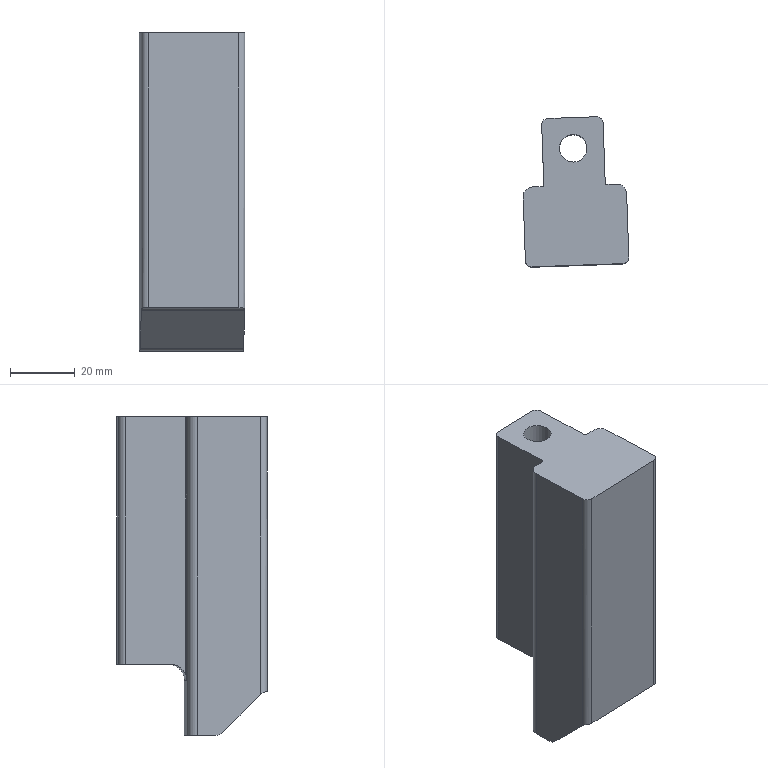Part | NX | features PU-10 2 | 1 solid | 25 faces | box 32.67 x 46.387 x 98.419 mm | volume 98260 mm3 | cylinder 13 | plane 12 | commonest cylinder face diameters 4 x4 6 x4 1 x2 8.506 x1 10 x1 14.5 x1
STEP:
#1=CARTESIAN_POINT('',(3512.219,-784.938,945.716));
#2=VERTEX_POINT('',#1);
#3=CARTESIAN_POINT('',(3512.07,-780.688,945.716));
#4=DIRECTION('',(0.,0.,-1.));
#5=DIRECTION('',(0.0349,-0.9994,0.));
#6=AXIS2_PLACEMENT_3D('',#3,#4,#5);
#7=CIRCLE('',#6,4.253);
#8=EDGE_CURVE('',#2,#2,#7,.F.);
#9=ORIENTED_EDGE('',*,*,#8,.T.);
#10=EDGE_LOOP('',(#9));
#11=FACE_BOUND('',#10,.T.);
#12=CARTESIAN_POINT('',(3511.922,-776.437,884.216));
#13=VERTEX_POINT('',#12);
#14=CARTESIAN_POINT('',(3512.07,-780.688,884.216));
#15=DIRECTION('',(0.,0.,1.));
#16=DIRECTION('',(1.,0.,0.));
#17=AXIS2_PLACEMENT_3D('',#14,#15,#16);
#18=CIRCLE('',#17,4.253);
#19=EDGE_CURVE('',#13,#13,#18,.T.);
#20=ORIENTED_EDGE('',*,*,#19,.F.);
#21=EDGE_LOOP('',(#20));
#22=FACE_BOUND('',#21,.T.);
#23=CARTESIAN_POINT('',(3512.07,-780.688,947.216));
#24=DIRECTION('',(0.,0.,-1.));
#25=DIRECTION('',(-0.0349,0.9994,0.));
#26=AXIS2_PLACEMENT_3D('',#23,#24,#25);
#27=CYLINDRICAL_SURFACE('',#26,4.253);
#28=ADVANCED_FACE('',(#11,#22),#27,.F.);
#29=CARTESIAN_POINT('',(3525.464,-791.727,945.716));
#30=VERTEX_POINT('',#29);
#31=CARTESIAN_POINT('',(3522.466,-791.832,945.716));
#32=VERTEX_POINT('',#31);
#33=CARTESIAN_POINT('',(3526.198,-791.701,945.716));
#34=DIRECTION('',(-0.9994,-0.0349,0.));
#35=VECTOR('',#34,1000.);
#36=LINE('',#33,#35);
#37=EDGE_CURVE('',#30,#32,#36,.T.);
#38=ORIENTED_EDGE('',*,*,#37,.T.);
#39=CARTESIAN_POINT('',(3521.948,-791.349,945.716));
#40=VERTEX_POINT('',#39);
#41=CARTESIAN_POINT('',(3522.448,-791.332,945.716));
#42=DIRECTION('',(0.,0.,-1.));
#43=DIRECTION('',(0.0349,-0.9994,0.));
#44=AXIS2_PLACEMENT_3D('',#41,#42,#43);
#45=CIRCLE('',#44,0.5);
#46=EDGE_CURVE('',#32,#40,#45,.T.);
#47=ORIENTED_EDGE('',*,*,#46,.T.);
#48=CARTESIAN_POINT('',(3521.303,-772.861,945.716));
#49=VERTEX_POINT('',#48);
#50=CARTESIAN_POINT('',(3521.966,-791.849,945.716));
#51=DIRECTION('',(0.0349,-0.9994,0.));
#52=VECTOR('',#51,1000.);
#53=LINE('',#50,#52);
#54=EDGE_CURVE('',#49,#40,#53,.T.);
#55=ORIENTED_EDGE('',*,*,#54,.F.);
#56=CARTESIAN_POINT('',(3519.234,-770.932,945.716));
#57=VERTEX_POINT('',#56);
#58=CARTESIAN_POINT('',(3519.304,-772.93,945.716));
#59=DIRECTION('',(0.,0.,-1.));
#60=DIRECTION('',(0.0349,-0.9994,0.));
#61=AXIS2_PLACEMENT_3D('',#58,#59,#60);
#62=CIRCLE('',#61,2.);
#63=EDGE_CURVE('',#49,#57,#62,.F.);
#64=ORIENTED_EDGE('',*,*,#63,.T.);
#65=CARTESIAN_POINT('',(3504.243,-771.455,945.716));
#66=VERTEX_POINT('',#65);
#67=CARTESIAN_POINT('',(3501.67,-771.545,945.716));
#68=DIRECTION('',(0.9994,0.0349,0.));
#69=VECTOR('',#68,1000.);
#70=LINE('',#67,#69);
#71=EDGE_CURVE('',#66,#57,#70,.T.);
#72=ORIENTED_EDGE('',*,*,#71,.F.);
#73=CARTESIAN_POINT('',(3502.314,-773.524,945.716));
#74=VERTEX_POINT('',#73);
#75=CARTESIAN_POINT('',(3504.313,-773.454,945.716));
#76=DIRECTION('',(0.,0.,-1.));
#77=DIRECTION('',(0.0349,-0.9994,0.));
#78=AXIS2_PLACEMENT_3D('',#75,#76,#77);
#79=CIRCLE('',#78,2.);
#80=EDGE_CURVE('',#66,#74,#79,.F.);
#81=ORIENTED_EDGE('',*,*,#80,.T.);
#82=CARTESIAN_POINT('',(3502.96,-792.012,945.716));
#83=VERTEX_POINT('',#82);
#84=CARTESIAN_POINT('',(3502.979,-792.562,945.716));
#85=DIRECTION('',(-0.0349,0.9994,0.));
#86=VECTOR('',#85,1000.);
#87=LINE('',#84,#86);
#88=EDGE_CURVE('',#83,#74,#87,.T.);
#89=ORIENTED_EDGE('',*,*,#88,.F.);
#90=CARTESIAN_POINT('',(3502.478,-792.53,945.716));
#91=VERTEX_POINT('',#90);
#92=CARTESIAN_POINT('',(3502.46,-792.03,945.716));
#93=DIRECTION('',(0.,0.,-1.));
#94=DIRECTION('',(0.0349,-0.9994,0.));
#95=AXIS2_PLACEMENT_3D('',#92,#93,#94);
#96=CIRCLE('',#95,0.5);
#97=EDGE_CURVE('',#83,#91,#96,.T.);
#98=ORIENTED_EDGE('',*,*,#97,.T.);
#99=CARTESIAN_POINT('',(3499.48,-792.634,945.716));
#100=VERTEX_POINT('',#99);
#101=CARTESIAN_POINT('',(3526.198,-791.701,945.716));
#102=DIRECTION('',(-0.9994,-0.0349,0.));
#103=VECTOR('',#102,1000.);
#104=LINE('',#101,#103);
#105=EDGE_CURVE('',#91,#100,#104,.T.);
#106=ORIENTED_EDGE('',*,*,#105,.T.);
#107=CARTESIAN_POINT('',(3496.586,-795.737,945.716));
#108=VERTEX_POINT('',#107);
#109=CARTESIAN_POINT('',(3499.584,-795.632,945.716));
#110=DIRECTION('',(0.,0.,-1.));
#111=DIRECTION('',(1.,0.,0.));
#112=AXIS2_PLACEMENT_3D('',#109,#110,#111);
#113=CIRCLE('',#112,3.);
#114=EDGE_CURVE('',#108,#100,#113,.T.);
#115=ORIENTED_EDGE('',*,*,#114,.F.);
#116=CARTESIAN_POINT('',(3497.272,-815.387,945.716));
#117=VERTEX_POINT('',#116);
#118=CARTESIAN_POINT('',(3497.206,-813.504,945.716));
#119=DIRECTION('',(0.0349,-0.9994,0.));
#120=VECTOR('',#119,1000.);
#121=LINE('',#118,#120);
#122=EDGE_CURVE('',#108,#117,#121,.T.);
#123=ORIENTED_EDGE('',*,*,#122,.T.);
#124=CARTESIAN_POINT('',(3499.341,-817.316,945.716));
#125=VERTEX_POINT('',#124);
#126=CARTESIAN_POINT('',(3499.271,-815.317,945.716));
#127=DIRECTION('',(0.,0.,-1.));
#128=DIRECTION('',(1.,0.,0.));
#129=AXIS2_PLACEMENT_3D('',#126,#127,#128);
#130=CIRCLE('',#129,2.);
#131=EDGE_CURVE('',#125,#117,#130,.T.);
#132=ORIENTED_EDGE('',*,*,#131,.F.);
#133=CARTESIAN_POINT('',(3527.324,-816.339,945.716));
#134=VERTEX_POINT('',#133);
#135=CARTESIAN_POINT('',(3551.474,-815.496,945.716));
#136=DIRECTION('',(0.9994,0.0349,0.));
#137=VECTOR('',#136,1000.);
#138=LINE('',#135,#137);
#139=EDGE_CURVE('',#125,#134,#138,.T.);
#140=ORIENTED_EDGE('',*,*,#139,.T.);
#141=CARTESIAN_POINT('',(3529.253,-814.27,945.716));
#142=VERTEX_POINT('',#141);
#143=CARTESIAN_POINT('',(3527.254,-814.34,945.716));
#144=DIRECTION('',(0.,0.,-1.));
#145=DIRECTION('',(1.,0.,0.));
#146=AXIS2_PLACEMENT_3D('',#143,#144,#145);
#147=CIRCLE('',#146,2.);
#148=EDGE_CURVE('',#142,#134,#147,.T.);
#149=ORIENTED_EDGE('',*,*,#148,.F.);
#150=CARTESIAN_POINT('',(3528.567,-794.62,945.716));
#151=VERTEX_POINT('',#150);
#152=CARTESIAN_POINT('',(3531.178,-869.419,945.716));
#153=DIRECTION('',(-0.0349,0.9994,0.));
#154=VECTOR('',#153,1000.);
#155=LINE('',#152,#154);
#156=EDGE_CURVE('',#142,#151,#155,.T.);
#157=ORIENTED_EDGE('',*,*,#156,.T.);
#158=CARTESIAN_POINT('',(3525.568,-794.725,945.716));
#159=DIRECTION('',(0.,0.,-1.));
#160=DIRECTION('',(1.,0.,0.));
#161=AXIS2_PLACEMENT_3D('',#158,#159,#160);
#162=CIRCLE('',#161,3.);
#163=EDGE_CURVE('',#30,#151,#162,.T.);
#164=ORIENTED_EDGE('',*,*,#163,.F.);
#165=EDGE_LOOP('',(#38,#47,#55,#64,#72,#81,#89,#98,#106,#115,#123,#132,#140,#149,#157,#164));
#166=FACE_BOUND('',#165,.T.);
#167=ORIENTED_EDGE('',*,*,#8,.F.);
#168=EDGE_LOOP('',(#167));
#169=FACE_BOUND('',#168,.T.);
#170=CARTESIAN_POINT('',(3897.665,-856.623,945.716));
#171=DIRECTION('',(0.,0.,1.));
#172=DIRECTION('',(1.,0.,0.));
#173=AXIS2_PLACEMENT_3D('',#170,#171,#172);
#174=PLANE('',#173);
#175=ADVANCED_FACE('',(#166,#169),#174,.T.);
#176=CARTESIAN_POINT('',(3499.48,-792.634,847.297));
#177=VERTEX_POINT('',#176);
#178=CARTESIAN_POINT('',(3499.48,-792.634,940.297));
#179=DIRECTION('',(0.,0.,-1.));
#180=VECTOR('',#179,1000.);
#181=LINE('',#178,#180);
#182=EDGE_CURVE('',#100,#177,#181,.T.);
#183=ORIENTED_EDGE('',*,*,#182,.T.);
#184=CARTESIAN_POINT('',(3496.586,-795.737,847.297));
#185=VERTEX_POINT('',#184);
#186=CARTESIAN_POINT('',(3499.584,-795.632,847.297));
#187=DIRECTION('',(-0.000000001,0.,1.));
#188=DIRECTION('',(-1.,0.,-0.000000001));
#189=AXIS2_PLACEMENT_3D('',#186,#187,#188);
#190=CIRCLE('',#189,3.);
#191=EDGE_CURVE('',#177,#185,#190,.T.);
#192=ORIENTED_EDGE('',*,*,#191,.T.);
#193=CARTESIAN_POINT('',(3496.586,-795.737,948.075));
#194=DIRECTION('',(0.,0.,-1.));
#195=VECTOR('',#194,1000.);
#196=LINE('',#193,#195);
#197=EDGE_CURVE('',#185,#108,#196,.F.);
#198=ORIENTED_EDGE('',*,*,#197,.T.);
#199=ORIENTED_EDGE('',*,*,#114,.T.);
#200=EDGE_LOOP('',(#183,#192,#198,#199));
#201=FACE_BOUND('',#200,.T.);
#202=CARTESIAN_POINT('',(3499.584,-795.632,940.297));
#203=DIRECTION('',(0.,0.,-1.));
#204=DIRECTION('',(-1.,0.,0.));
#205=AXIS2_PLACEMENT_3D('',#202,#203,#204);
#206=CYLINDRICAL_SURFACE('',#205,3.);
#207=ADVANCED_FACE('',(#201),#206,.T.);
#208=CARTESIAN_POINT('',(3497.272,-815.387,859.952));
#209=VERTEX_POINT('',#208);
#210=CARTESIAN_POINT('',(3497.272,-815.387,948.075));
#211=DIRECTION('',(0.,0.,-1.));
#212=VECTOR('',#211,1000.);
#213=LINE('',#210,#212);
#214=EDGE_CURVE('',#117,#209,#213,.T.);
#215=ORIENTED_EDGE('',*,*,#214,.T.);
#216=CARTESIAN_POINT('',(3499.341,-817.316,860.716));
#217=VERTEX_POINT('',#216);
#218=CARTESIAN_POINT('',(3497.272,-815.387,859.952));
#219=CARTESIAN_POINT('',(3497.287,-815.802,860.324));
#220=CARTESIAN_POINT('',(3497.652,-816.867,860.77));
#221=CARTESIAN_POINT('',(3498.783,-817.335,860.716));
#222=CARTESIAN_POINT('',(3499.341,-817.316,860.716));
#223=B_SPLINE_CURVE_WITH_KNOTS('',3,(#218,#219,#220,#221,#222),.UNSPECIFIED.,.F.,.F.,(4,1,4),(0.,0.001653,0.003307),.UNSPECIFIED.);
#224=EDGE_CURVE('',#209,#217,#223,.T.);
#225=ORIENTED_EDGE('',*,*,#224,.T.);
#226=CARTESIAN_POINT('',(3499.341,-817.316,950.716));
#227=DIRECTION('',(0.,0.,-1.));
#228=VECTOR('',#227,1000.);
#229=LINE('',#226,#228);
#230=EDGE_CURVE('',#217,#125,#229,.F.);
#231=ORIENTED_EDGE('',*,*,#230,.T.);
#232=ORIENTED_EDGE('',*,*,#131,.T.);
#233=EDGE_LOOP('',(#215,#225,#231,#232));
#234=FACE_BOUND('',#233,.T.);
#235=CARTESIAN_POINT('',(3499.271,-815.317,948.075));
#236=DIRECTION('',(0.,0.,-1.));
#237=DIRECTION('',(-1.,0.,0.));
#238=AXIS2_PLACEMENT_3D('',#235,#236,#237);
#239=CYLINDRICAL_SURFACE('',#238,2.);
#240=ADVANCED_FACE('',(#234),#239,.T.);
#241=ORIENTED_EDGE('',*,*,#197,.F.);
#242=CARTESIAN_POINT('',(3496.787,-801.491,847.297));
#243=VERTEX_POINT('',#242);
#244=CARTESIAN_POINT('',(3496.656,-797.736,847.297));
#245=DIRECTION('',(0.0349,-0.9994,0.));
#246=VECTOR('',#245,1000.);
#247=LINE('',#244,#246);
#248=EDGE_CURVE('',#185,#243,#247,.T.);
#249=ORIENTED_EDGE('',*,*,#248,.T.);
#250=CARTESIAN_POINT('',(3496.861,-803.611,848.176));
#251=VERTEX_POINT('',#250);
#252=CARTESIAN_POINT('',(3496.787,-801.491,850.297));
#253=DIRECTION('',(-0.9994,-0.0349,0.));
#254=DIRECTION('',(0.0349,-0.9994,0.));
#255=AXIS2_PLACEMENT_3D('',#252,#253,#254);
#256=CIRCLE('',#255,3.);
#257=EDGE_CURVE('',#243,#251,#256,.T.);
#258=ORIENTED_EDGE('',*,*,#257,.T.);
#259=CARTESIAN_POINT('',(3497.268,-815.266,859.838));
#260=VERTEX_POINT('',#259);
#261=CARTESIAN_POINT('',(3498.777,-858.477,903.075));
#262=DIRECTION('',(0.02467,-0.7067,0.7071));
#263=VECTOR('',#262,1000.);
#264=LINE('',#261,#263);
#265=EDGE_CURVE('',#251,#260,#264,.T.);
#266=ORIENTED_EDGE('',*,*,#265,.T.);
#267=CARTESIAN_POINT('',(3497.342,-817.386,857.716));
#268=DIRECTION('',(0.9994,0.0349,0.));
#269=DIRECTION('',(-0.0349,0.9994,0.));
#270=AXIS2_PLACEMENT_3D('',#267,#268,#269);
#271=CIRCLE('',#270,3.);
#272=EDGE_CURVE('',#260,#209,#271,.T.);
#273=ORIENTED_EDGE('',*,*,#272,.T.);
#274=ORIENTED_EDGE('',*,*,#214,.F.);
#275=ORIENTED_EDGE('',*,*,#122,.F.);
#276=EDGE_LOOP('',(#241,#249,#258,#266,#273,#274,#275));
#277=FACE_BOUND('',#276,.T.);
#278=CARTESIAN_POINT('',(3497.206,-813.504,948.075));
#279=DIRECTION('',(-0.9994,-0.0349,0.));
#280=DIRECTION('',(-0.0349,0.9994,0.));
#281=AXIS2_PLACEMENT_3D('',#278,#279,#280);
#282=PLANE('',#281);
#283=ADVANCED_FACE('',(#277),#282,.T.);
#284=CARTESIAN_POINT('',(3528.567,-794.62,847.297));
#285=VERTEX_POINT('',#284);
#286=CARTESIAN_POINT('',(3528.567,-794.62,849.297));
#287=DIRECTION('',(0.,0.,-1.));
#288=VECTOR('',#287,1000.);
#289=LINE('',#286,#288);
#290=EDGE_CURVE('',#151,#285,#289,.T.);
#291=ORIENTED_EDGE('',*,*,#290,.T.);
#292=CARTESIAN_POINT('',(3525.464,-791.727,847.297));
#293=VERTEX_POINT('',#292);
#294=CARTESIAN_POINT('',(3525.568,-794.725,847.297));
#295=DIRECTION('',(-0.000000001,0.,1.));
#296=DIRECTION('',(-1.,0.,-0.000000001));
#297=AXIS2_PLACEMENT_3D('',#294,#295,#296);
#298=CIRCLE('',#297,3.);
#299=EDGE_CURVE('',#285,#293,#298,.T.);
#300=ORIENTED_EDGE('',*,*,#299,.T.);
#301=CARTESIAN_POINT('',(3525.464,-791.727,935.716));
#302=DIRECTION('',(0.,0.,-1.));
#303=VECTOR('',#302,1000.);
#304=LINE('',#301,#303);
#305=EDGE_CURVE('',#293,#30,#304,.F.);
#306=ORIENTED_EDGE('',*,*,#305,.T.);
#307=ORIENTED_EDGE('',*,*,#163,.T.);
#308=EDGE_LOOP('',(#291,#300,#306,#307));
#309=FACE_BOUND('',#308,.T.);
#310=CARTESIAN_POINT('',(3525.568,-794.725,891.507));
#311=DIRECTION('',(0.,0.,1.));
#312=DIRECTION('',(1.,0.,0.));
#313=AXIS2_PLACEMENT_3D('',#310,#311,#312);
#314=CYLINDRICAL_SURFACE('',#313,3.);
#315=ADVANCED_FACE('',(#309),#314,.T.);
#316=CARTESIAN_POINT('',(3527.324,-816.339,860.716));
#317=VERTEX_POINT('',#316);
#318=CARTESIAN_POINT('',(3527.324,-816.339,860.716));
#319=DIRECTION('',(0.,0.,-1.));
#320=VECTOR('',#319,1000.);
#321=LINE('',#318,#320);
#322=EDGE_CURVE('',#134,#317,#321,.T.);
#323=ORIENTED_EDGE('',*,*,#322,.T.);
#324=CARTESIAN_POINT('',(3529.253,-814.27,859.952));
#325=VERTEX_POINT('',#324);
#326=CARTESIAN_POINT('',(3527.324,-816.339,860.716));
#327=CARTESIAN_POINT('',(3527.882,-816.319,860.716));
#328=CARTESIAN_POINT('',(3528.973,-815.777,860.771));
#329=CARTESIAN_POINT('',(3529.267,-814.686,860.325));
#330=CARTESIAN_POINT('',(3529.253,-814.27,859.952));
#331=B_SPLINE_CURVE_WITH_KNOTS('',3,(#326,#327,#328,#329,#330),.UNSPECIFIED.,.F.,.F.,(4,1,4),(0.,0.001652,0.003305),.UNSPECIFIED.);
#332=EDGE_CURVE('',#317,#325,#331,.T.);
#333=ORIENTED_EDGE('',*,*,#332,.T.);
#334=CARTESIAN_POINT('',(3529.253,-814.27,935.716));
#335=DIRECTION('',(0.,0.,-1.));
#336=VECTOR('',#335,1000.);
#337=LINE('',#334,#336);
#338=EDGE_CURVE('',#325,#142,#337,.F.);
#339=ORIENTED_EDGE('',*,*,#338,.T.);
#340=ORIENTED_EDGE('',*,*,#148,.T.);
#341=EDGE_LOOP('',(#323,#333,#339,#340));
#342=FACE_BOUND('',#341,.T.);
#343=CARTESIAN_POINT('',(3527.254,-814.34,950.716));
#344=DIRECTION('',(0.,0.,1.));
#345=DIRECTION('',(1.,0.,0.));
#346=AXIS2_PLACEMENT_3D('',#343,#344,#345);
#347=CYLINDRICAL_SURFACE('',#346,2.);
#348=ADVANCED_FACE('',(#342),#347,.T.);
#349=ORIENTED_EDGE('',*,*,#338,.F.);
#350=CARTESIAN_POINT('',(3529.248,-814.149,859.838));
#351=VERTEX_POINT('',#350);
#352=CARTESIAN_POINT('',(3529.323,-816.269,857.716));
#353=DIRECTION('',(0.9994,0.0349,0.));
#354=DIRECTION('',(-0.0349,0.9994,0.));
#355=AXIS2_PLACEMENT_3D('',#352,#353,#354);
#356=CIRCLE('',#355,3.);
#357=EDGE_CURVE('',#351,#325,#356,.T.);
#358=ORIENTED_EDGE('',*,*,#357,.F.);
#359=CARTESIAN_POINT('',(3528.842,-802.494,848.176));
#360=VERTEX_POINT('',#359);
#361=CARTESIAN_POINT('',(3529.138,-810.991,856.678));
#362=DIRECTION('',(-0.02467,0.7067,-0.7071));
#363=VECTOR('',#362,1000.);
#364=LINE('',#361,#363);
#365=EDGE_CURVE('',#351,#360,#364,.T.);
#366=ORIENTED_EDGE('',*,*,#365,.T.);
#367=CARTESIAN_POINT('',(3528.768,-800.374,847.297));
#368=VERTEX_POINT('',#367);
#369=CARTESIAN_POINT('',(3528.768,-800.374,850.297));
#370=DIRECTION('',(-0.9994,-0.0349,0.));
#371=DIRECTION('',(0.0349,-0.9994,0.));
#372=AXIS2_PLACEMENT_3D('',#369,#370,#371);
#373=CIRCLE('',#372,3.);
#374=EDGE_CURVE('',#360,#368,#373,.F.);
#375=ORIENTED_EDGE('',*,*,#374,.T.);
#376=CARTESIAN_POINT('',(3528.636,-796.619,847.297));
#377=DIRECTION('',(0.0349,-0.9994,0.));
#378=VECTOR('',#377,1000.);
#379=LINE('',#376,#378);
#380=EDGE_CURVE('',#285,#368,#379,.T.);
#381=ORIENTED_EDGE('',*,*,#380,.F.);
#382=ORIENTED_EDGE('',*,*,#290,.F.);
#383=ORIENTED_EDGE('',*,*,#156,.F.);
#384=EDGE_LOOP('',(#349,#358,#366,#375,#381,#382,#383));
#385=FACE_BOUND('',#384,.T.);
#386=CARTESIAN_POINT('',(3528.98,-806.471,891.507));
#387=DIRECTION('',(-0.9994,-0.0349,0.));
#388=DIRECTION('',(-0.0349,0.9994,0.));
#389=AXIS2_PLACEMENT_3D('',#386,#387,#388);
#390=PLANE('',#389);
#391=ADVANCED_FACE('',(#385),#390,.F.);
#392=ORIENTED_EDGE('',*,*,#230,.F.);
#393=CARTESIAN_POINT('',(3527.324,-816.339,860.716));
#394=CARTESIAN_POINT('',(3517.996,-816.664,860.716));
#395=CARTESIAN_POINT('',(3508.668,-816.99,860.716));
#396=CARTESIAN_POINT('',(3499.341,-817.316,860.716));
#397=B_SPLINE_CURVE_WITH_KNOTS('',3,(#393,#394,#395,#396),.UNSPECIFIED.,.F.,.F.,(4,4),(0.0342,0.9964),.UNSPECIFIED.);
#398=EDGE_CURVE('',#217,#317,#397,.F.);
#399=ORIENTED_EDGE('',*,*,#398,.T.);
#400=ORIENTED_EDGE('',*,*,#322,.F.);
#401=ORIENTED_EDGE('',*,*,#139,.F.);
#402=EDGE_LOOP('',(#392,#399,#400,#401));
#403=FACE_BOUND('',#402,.T.);
#404=CARTESIAN_POINT('',(3551.474,-815.496,950.716));
#405=DIRECTION('',(0.0349,-0.9994,0.));
#406=DIRECTION('',(-0.9994,-0.0349,0.));
#407=AXIS2_PLACEMENT_3D('',#404,#405,#406);
#408=PLANE('',#407);
#409=ADVANCED_FACE('',(#403),#408,.T.);
#410=CARTESIAN_POINT('',(3502.96,-792.012,866.396));
#411=VERTEX_POINT('',#410);
#412=CARTESIAN_POINT('',(3502.96,-792.012,937.216));
#413=DIRECTION('',(0.,0.,1.));
#414=VECTOR('',#413,1000.);
#415=LINE('',#412,#414);
#416=EDGE_CURVE('',#411,#83,#415,.T.);
#417=ORIENTED_EDGE('',*,*,#416,.F.);
#418=CARTESIAN_POINT('',(3502.478,-792.53,864.217));
#419=VERTEX_POINT('',#418);
#420=CARTESIAN_POINT('',(3502.96,-792.012,866.396));
#421=CARTESIAN_POINT('',(3502.972,-792.353,865.693));
#422=CARTESIAN_POINT('',(3502.71,-792.521,864.951));
#423=CARTESIAN_POINT('',(3502.478,-792.53,864.217));
#424=B_SPLINE_CURVE_WITH_KNOTS('',3,(#420,#421,#422,#423),.UNSPECIFIED.,.F.,.F.,(4,4),(0.,0.002312),.UNSPECIFIED.);
#425=EDGE_CURVE('',#411,#419,#424,.T.);
#426=ORIENTED_EDGE('',*,*,#425,.T.);
#427=CARTESIAN_POINT('',(3502.478,-792.53,895.217));
#428=DIRECTION('',(0.,0.,-1.));
#429=VECTOR('',#428,1000.);
#430=LINE('',#427,#429);
#431=EDGE_CURVE('',#91,#419,#430,.T.);
#432=ORIENTED_EDGE('',*,*,#431,.F.);
#433=ORIENTED_EDGE('',*,*,#97,.F.);
#434=EDGE_LOOP('',(#417,#426,#432,#433));
#435=FACE_BOUND('',#434,.T.);
#436=CARTESIAN_POINT('',(3502.46,-792.03,929.216));
#437=DIRECTION('',(0.,0.,-1.));
#438=DIRECTION('',(-0.0349,0.9994,0.));
#439=AXIS2_PLACEMENT_3D('',#436,#437,#438);
#440=CYLINDRICAL_SURFACE('',#439,0.5);
#441=ADVANCED_FACE('',(#435),#440,.F.);
#442=CARTESIAN_POINT('',(3502.314,-773.524,869.217));
#443=VERTEX_POINT('',#442);
#444=CARTESIAN_POINT('',(3502.314,-773.524,929.216));
#445=DIRECTION('',(0.,0.,-1.));
#446=VECTOR('',#445,1000.);
#447=LINE('',#444,#446);
#448=EDGE_CURVE('',#74,#443,#447,.T.);
#449=ORIENTED_EDGE('',*,*,#448,.T.);
#450=CARTESIAN_POINT('',(3502.803,-787.515,869.217));
#451=VERTEX_POINT('',#450);
#452=CARTESIAN_POINT('',(3498.279,-657.945,869.217));
#453=DIRECTION('',(-0.0349,0.9994,0.));
#454=VECTOR('',#453,1000.);
#455=LINE('',#452,#454);
#456=EDGE_CURVE('',#451,#443,#455,.T.);
#457=ORIENTED_EDGE('',*,*,#456,.F.);
#458=CARTESIAN_POINT('',(3502.803,-787.515,864.217));
#459=DIRECTION('',(0.9994,0.0349,0.));
#460=DIRECTION('',(-0.0349,0.9994,0.));
#461=AXIS2_PLACEMENT_3D('',#458,#459,#460);
#462=CIRCLE('',#461,5.);
#463=EDGE_CURVE('',#451,#411,#462,.T.);
#464=ORIENTED_EDGE('',*,*,#463,.T.);
#465=ORIENTED_EDGE('',*,*,#416,.T.);
#466=ORIENTED_EDGE('',*,*,#88,.T.);
#467=EDGE_LOOP('',(#449,#457,#464,#465,#466));
#468=FACE_BOUND('',#467,.T.);
#469=CARTESIAN_POINT('',(3502.979,-792.562,929.216));
#470=DIRECTION('',(0.9994,0.0349,0.));
#471=DIRECTION('',(0.,0.,-1.));
#472=AXIS2_PLACEMENT_3D('',#469,#470,#471);
#473=PLANE('',#472);
#474=ADVANCED_FACE('',(#468),#473,.F.);
#475=CARTESIAN_POINT('',(3504.243,-771.455,869.217));
#476=VERTEX_POINT('',#475);
#477=CARTESIAN_POINT('',(3504.243,-771.455,929.216));
#478=DIRECTION('',(0.,0.,1.));
#479=VECTOR('',#478,1000.);
#480=LINE('',#477,#479);
#481=EDGE_CURVE('',#476,#66,#480,.T.);
#482=ORIENTED_EDGE('',*,*,#481,.F.);
#483=CARTESIAN_POINT('',(3504.313,-773.454,869.217));
#484=DIRECTION('',(0.,0.,-1.));
#485=DIRECTION('',(0.0349,-0.9994,0.));
#486=AXIS2_PLACEMENT_3D('',#483,#484,#485);
#487=CIRCLE('',#486,2.);
#488=EDGE_CURVE('',#443,#476,#487,.T.);
#489=ORIENTED_EDGE('',*,*,#488,.F.);
#490=ORIENTED_EDGE('',*,*,#448,.F.);
#491=ORIENTED_EDGE('',*,*,#80,.F.);
#492=EDGE_LOOP('',(#482,#489,#490,#491));
#493=FACE_BOUND('',#492,.T.);
#494=CARTESIAN_POINT('',(3504.313,-773.454,929.216));
#495=DIRECTION('',(0.,0.,-1.));
#496=DIRECTION('',(-0.0349,0.9994,0.));
#497=AXIS2_PLACEMENT_3D('',#494,#495,#496);
#498=CYLINDRICAL_SURFACE('',#497,2.);
#499=ADVANCED_FACE('',(#493),#498,.T.);
#500=CARTESIAN_POINT('',(3519.234,-770.932,869.217));
#501=VERTEX_POINT('',#500);
#502=CARTESIAN_POINT('',(3519.234,-770.932,929.216));
#503=DIRECTION('',(0.,0.,-1.));
#504=VECTOR('',#503,1000.);
#505=LINE('',#502,#504);
#506=EDGE_CURVE('',#57,#501,#505,.T.);
#507=ORIENTED_EDGE('',*,*,#506,.T.);
#508=CARTESIAN_POINT('',(2766.196,-797.225,869.217));
#509=DIRECTION('',(0.9994,0.0349,0.));
#510=VECTOR('',#509,1000.);
#511=LINE('',#508,#510);
#512=EDGE_CURVE('',#476,#501,#511,.T.);
#513=ORIENTED_EDGE('',*,*,#512,.F.);
#514=ORIENTED_EDGE('',*,*,#481,.T.);
#515=ORIENTED_EDGE('',*,*,#71,.T.);
#516=EDGE_LOOP('',(#507,#513,#514,#515));
#517=FACE_BOUND('',#516,.T.);
#518=CARTESIAN_POINT('',(3501.67,-771.545,929.216));
#519=DIRECTION('',(0.0349,-0.9994,0.));
#520=DIRECTION('',(0.,0.,1.));
#521=AXIS2_PLACEMENT_3D('',#518,#519,#520);
#522=PLANE('',#521);
#523=ADVANCED_FACE('',(#517),#522,.F.);
#524=CARTESIAN_POINT('',(3521.303,-772.861,869.217));
#525=VERTEX_POINT('',#524);
#526=CARTESIAN_POINT('',(3521.303,-772.861,929.216));
#527=DIRECTION('',(0.,0.,1.));
#528=VECTOR('',#527,1000.);
#529=LINE('',#526,#528);
#530=EDGE_CURVE('',#525,#49,#529,.T.);
#531=ORIENTED_EDGE('',*,*,#530,.F.);
#532=CARTESIAN_POINT('',(3519.304,-772.93,869.217));
#533=DIRECTION('',(0.,0.,-1.));
#534=DIRECTION('',(0.0349,-0.9994,0.));
#535=AXIS2_PLACEMENT_3D('',#532,#533,#534);
#536=CIRCLE('',#535,2.);
#537=EDGE_CURVE('',#501,#525,#536,.T.);
#538=ORIENTED_EDGE('',*,*,#537,.F.);
#539=ORIENTED_EDGE('',*,*,#506,.F.);
#540=ORIENTED_EDGE('',*,*,#63,.F.);
#541=EDGE_LOOP('',(#531,#538,#539,#540));
#542=FACE_BOUND('',#541,.T.);
#543=CARTESIAN_POINT('',(3519.304,-772.93,929.216));
#544=DIRECTION('',(0.,0.,1.));
#545=DIRECTION('',(0.0349,-0.9994,0.));
#546=AXIS2_PLACEMENT_3D('',#543,#544,#545);
#547=CYLINDRICAL_SURFACE('',#546,2.);
#548=ADVANCED_FACE('',(#542),#547,.T.);
#549=CARTESIAN_POINT('',(3522.466,-791.832,864.217));
#550=VERTEX_POINT('',#549);
#551=CARTESIAN_POINT('',(3522.466,-791.832,937.216));
#552=DIRECTION('',(0.,0.,1.));
#553=VECTOR('',#552,1000.);
#554=LINE('',#551,#553);
#555=EDGE_CURVE('',#550,#32,#554,.T.);
#556=ORIENTED_EDGE('',*,*,#555,.F.);
#557=CARTESIAN_POINT('',(3521.948,-791.349,866.396));
#558=VERTEX_POINT('',#557);
#559=CARTESIAN_POINT('',(3521.948,-791.349,866.396));
#560=CARTESIAN_POINT('',(3521.96,-791.69,865.693));
#561=CARTESIAN_POINT('',(3522.233,-791.84,864.951));
#562=CARTESIAN_POINT('',(3522.466,-791.832,864.217));
#563=B_SPLINE_CURVE_WITH_KNOTS('',3,(#559,#560,#561,#562),.UNSPECIFIED.,.F.,.F.,(4,4),(0.,0.002312),.UNSPECIFIED.);
#564=EDGE_CURVE('',#550,#558,#563,.F.);
#565=ORIENTED_EDGE('',*,*,#564,.T.);
#566=CARTESIAN_POINT('',(3521.948,-791.349,895.217));
#567=DIRECTION('',(0.,0.,-1.));
#568=VECTOR('',#567,1000.);
#569=LINE('',#566,#568);
#570=EDGE_CURVE('',#40,#558,#569,.T.);
#571=ORIENTED_EDGE('',*,*,#570,.F.);
#572=ORIENTED_EDGE('',*,*,#46,.F.);
#573=EDGE_LOOP('',(#556,#565,#571,#572));
#574=FACE_BOUND('',#573,.T.);
#575=CARTESIAN_POINT('',(3522.448,-791.332,929.216));
#576=DIRECTION('',(0.,0.,1.));
#577=DIRECTION('',(0.0349,-0.9994,0.));
#578=AXIS2_PLACEMENT_3D('',#575,#576,#577);
#579=CYLINDRICAL_SURFACE('',#578,0.5);
#580=ADVANCED_FACE('',(#574),#579,.F.);
#581=ORIENTED_EDGE('',*,*,#570,.T.);
#582=CARTESIAN_POINT('',(3521.791,-786.852,869.217));
#583=VERTEX_POINT('',#582);
#584=CARTESIAN_POINT('',(3521.791,-786.852,864.217));
#585=DIRECTION('',(-0.9994,-0.0349,0.));
#586=DIRECTION('',(0.0349,-0.9994,0.));
#587=AXIS2_PLACEMENT_3D('',#584,#585,#586);
#588=CIRCLE('',#587,5.);
#589=EDGE_CURVE('',#558,#583,#588,.T.);
#590=ORIENTED_EDGE('',*,*,#589,.T.);
#591=CARTESIAN_POINT('',(3517.267,-657.282,869.217));
#592=DIRECTION('',(0.0349,-0.9994,0.));
#593=VECTOR('',#592,1000.);
#594=LINE('',#591,#593);
#595=EDGE_CURVE('',#525,#583,#594,.T.);
#596=ORIENTED_EDGE('',*,*,#595,.F.);
#597=ORIENTED_EDGE('',*,*,#530,.T.);
#598=ORIENTED_EDGE('',*,*,#54,.T.);
#599=EDGE_LOOP('',(#581,#590,#596,#597,#598));
#600=FACE_BOUND('',#599,.T.);
#601=CARTESIAN_POINT('',(3521.966,-791.849,929.216));
#602=DIRECTION('',(-0.9994,-0.0349,0.));
#603=DIRECTION('',(0.,0.,1.));
#604=AXIS2_PLACEMENT_3D('',#601,#602,#603);
#605=PLANE('',#604);
#606=ADVANCED_FACE('',(#600),#605,.F.);
#607=ORIENTED_EDGE('',*,*,#305,.F.);
#608=CARTESIAN_POINT('',(3526.198,-791.701,847.297));
#609=DIRECTION('',(0.9994,0.0349,0.000000001));
#610=VECTOR('',#609,1000.);
#611=LINE('',#608,#610);
#612=EDGE_CURVE('',#177,#293,#611,.T.);
#613=ORIENTED_EDGE('',*,*,#612,.F.);
#614=ORIENTED_EDGE('',*,*,#182,.F.);
#615=ORIENTED_EDGE('',*,*,#105,.F.);
#616=ORIENTED_EDGE('',*,*,#431,.T.);
#617=CARTESIAN_POINT('',(2766.928,-818.212,864.217));
#618=DIRECTION('',(-0.9994,-0.0349,0.));
#619=VECTOR('',#618,1000.);
#620=LINE('',#617,#619);
#621=EDGE_CURVE('',#419,#550,#620,.F.);
#622=ORIENTED_EDGE('',*,*,#621,.T.);
#623=ORIENTED_EDGE('',*,*,#555,.T.);
#624=ORIENTED_EDGE('',*,*,#37,.F.);
#625=EDGE_LOOP('',(#607,#613,#614,#615,#616,#622,#623,#624));
#626=FACE_BOUND('',#625,.T.);
#627=CARTESIAN_POINT('',(3526.198,-791.701,940.297));
#628=DIRECTION('',(-0.0349,0.9994,0.));
#629=DIRECTION('',(0.9994,0.0349,0.));
#630=AXIS2_PLACEMENT_3D('',#627,#628,#629);
#631=PLANE('',#630);
#632=ADVANCED_FACE('',(#626),#631,.T.);
#633=ORIENTED_EDGE('',*,*,#265,.F.);
#634=CARTESIAN_POINT('',(3528.842,-802.494,848.176));
#635=DIRECTION('',(-0.9994,-0.0349,-0.000000001));
#636=VECTOR('',#635,1000.);
#637=LINE('',#634,#636);
#638=EDGE_CURVE('',#251,#360,#637,.F.);
#639=ORIENTED_EDGE('',*,*,#638,.T.);
#640=ORIENTED_EDGE('',*,*,#365,.F.);
#641=CARTESIAN_POINT('',(3551.4,-813.376,859.838));
#642=DIRECTION('',(0.9994,0.0349,0.));
#643=VECTOR('',#642,1000.);
#644=LINE('',#641,#643);
#645=EDGE_CURVE('',#260,#351,#644,.T.);
#646=ORIENTED_EDGE('',*,*,#645,.F.);
#647=EDGE_LOOP('',(#633,#639,#640,#646));
#648=FACE_BOUND('',#647,.T.);
#649=CARTESIAN_POINT('',(3551.289,-810.217,856.678));
#650=DIRECTION('',(-0.02467,0.7067,0.7071));
#651=DIRECTION('',(0.02467,-0.7067,0.7071));
#652=AXIS2_PLACEMENT_3D('',#649,#650,#651);
#653=PLANE('',#652);
#654=ADVANCED_FACE('',(#648),#653,.F.);
#655=ORIENTED_EDGE('',*,*,#272,.F.);
#656=ORIENTED_EDGE('',*,*,#645,.T.);
#657=ORIENTED_EDGE('',*,*,#357,.T.);
#658=ORIENTED_EDGE('',*,*,#332,.F.);
#659=ORIENTED_EDGE('',*,*,#398,.F.);
#660=ORIENTED_EDGE('',*,*,#224,.F.);
#661=EDGE_LOOP('',(#655,#656,#657,#658,#659,#660));
#662=FACE_BOUND('',#661,.T.);
#663=CARTESIAN_POINT('',(3551.474,-815.496,857.716));
#664=DIRECTION('',(0.9994,0.0349,0.));
#665=DIRECTION('',(-0.0349,0.9994,0.));
#666=AXIS2_PLACEMENT_3D('',#663,#664,#665);
#667=CYLINDRICAL_SURFACE('',#666,3.);
#668=ADVANCED_FACE('',(#662),#667,.F.);
#669=ORIENTED_EDGE('',*,*,#380,.T.);
#670=CARTESIAN_POINT('',(3496.787,-801.491,847.297));
#671=DIRECTION('',(-0.9994,-0.0349,-0.000000001));
#672=VECTOR('',#671,1000.);
#673=LINE('',#670,#672);
#674=EDGE_CURVE('',#368,#243,#673,.T.);
#675=ORIENTED_EDGE('',*,*,#674,.T.);
#676=ORIENTED_EDGE('',*,*,#248,.F.);
#677=ORIENTED_EDGE('',*,*,#191,.F.);
#678=ORIENTED_EDGE('',*,*,#612,.T.);
#679=ORIENTED_EDGE('',*,*,#299,.F.);
#680=EDGE_LOOP('',(#669,#675,#676,#677,#678,#679));
#681=FACE_BOUND('',#680,.T.);
#682=CARTESIAN_POINT('',(3526.372,-796.698,847.297));
#683=DIRECTION('',(0.000000001,0.,-1.));
#684=DIRECTION('',(-1.,0.,-0.000000001));
#685=AXIS2_PLACEMENT_3D('',#682,#683,#684);
#686=PLANE('',#685);
#687=ADVANCED_FACE('',(#681),#686,.T.);
#688=ORIENTED_EDGE('',*,*,#374,.F.);
#689=ORIENTED_EDGE('',*,*,#638,.F.);
#690=ORIENTED_EDGE('',*,*,#257,.F.);
#691=ORIENTED_EDGE('',*,*,#674,.F.);
#692=EDGE_LOOP('',(#688,#689,#690,#691));
#693=FACE_BOUND('',#692,.T.);
#694=CARTESIAN_POINT('',(3526.503,-800.453,850.297));
#695=DIRECTION('',(0.9994,0.0349,0.000000001));
#696=DIRECTION('',(-0.0349,0.9994,0.));
#697=AXIS2_PLACEMENT_3D('',#694,#695,#696);
#698=CYLINDRICAL_SURFACE('',#697,3.);
#699=ADVANCED_FACE('',(#693),#698,.T.);
#700=CARTESIAN_POINT('',(3509.088,-787.296,869.217));
#701=VERTEX_POINT('',#700);
#702=CARTESIAN_POINT('',(3515.507,-787.072,869.217));
#703=VERTEX_POINT('',#702);
#704=CARTESIAN_POINT('',(3509.088,-787.296,869.217));
#705=CARTESIAN_POINT('',(3510.108,-787.756,869.217));
#706=CARTESIAN_POINT('',(3512.326,-788.188,869.103));
#707=CARTESIAN_POINT('',(3514.521,-787.602,869.217));
#708=CARTESIAN_POINT('',(3515.507,-787.072,869.217));
#709=B_SPLINE_CURVE_WITH_KNOTS('',3,(#704,#705,#706,#707,#708),.UNSPECIFIED.,.F.,.F.,(4,1,4),(0.,0.003304,0.006609),.UNSPECIFIED.);
#710=EDGE_CURVE('',#701,#703,#709,.T.);
#711=ORIENTED_EDGE('',*,*,#710,.F.);
#712=CARTESIAN_POINT('',(3512.07,-780.688,869.217));
#713=DIRECTION('',(0.,0.,1.));
#714=DIRECTION('',(0.0349,-0.9994,0.));
#715=AXIS2_PLACEMENT_3D('',#712,#713,#714);
#716=CIRCLE('',#715,7.25);
#717=EDGE_CURVE('',#703,#701,#716,.T.);
#718=ORIENTED_EDGE('',*,*,#717,.F.);
#719=EDGE_LOOP('',(#711,#718));
#720=FACE_BOUND('',#719,.T.);
#721=CARTESIAN_POINT('',(3511.817,-773.442,884.216));
#722=VERTEX_POINT('',#721);
#723=CARTESIAN_POINT('',(3512.07,-780.688,884.216));
#724=DIRECTION('',(0.,0.,1.));
#725=DIRECTION('',(1.,0.,0.));
#726=AXIS2_PLACEMENT_3D('',#723,#724,#725);
#727=CIRCLE('',#726,7.25);
#728=EDGE_CURVE('',#722,#722,#727,.F.);
#729=ORIENTED_EDGE('',*,*,#728,.F.);
#730=EDGE_LOOP('',(#729));
#731=FACE_BOUND('',#730,.T.);
#732=CARTESIAN_POINT('',(3512.07,-780.688,912.216));
#733=DIRECTION('',(0.,0.,-1.));
#734=DIRECTION('',(-0.0349,0.9994,0.));
#735=AXIS2_PLACEMENT_3D('',#732,#733,#734);
#736=CYLINDRICAL_SURFACE('',#735,7.25);
#737=ADVANCED_FACE('',(#720,#731),#736,.F.);
#738=ORIENTED_EDGE('',*,*,#19,.T.);
#739=EDGE_LOOP('',(#738));
#740=FACE_BOUND('',#739,.T.);
#741=ORIENTED_EDGE('',*,*,#728,.T.);
#742=EDGE_LOOP('',(#741));
#743=FACE_BOUND('',#742,.T.);
#744=CARTESIAN_POINT('',(3437.678,-309.966,884.216));
#745=DIRECTION('',(0.,0.,1.));
#746=DIRECTION('',(0.0349,-0.9994,0.));
#747=AXIS2_PLACEMENT_3D('',#744,#745,#746);
#748=PLANE('',#747);
#749=ADVANCED_FACE('',(#740,#743),#748,.F.);
#750=ORIENTED_EDGE('',*,*,#595,.T.);
#751=CARTESIAN_POINT('',(3502.303,-787.533,869.217));
#752=DIRECTION('',(-0.9994,-0.0349,0.));
#753=VECTOR('',#752,1000.);
#754=LINE('',#751,#753);
#755=EDGE_CURVE('',#583,#703,#754,.T.);
#756=ORIENTED_EDGE('',*,*,#755,.T.);
#757=ORIENTED_EDGE('',*,*,#717,.T.);
#758=CARTESIAN_POINT('',(3502.303,-787.533,869.217));
#759=DIRECTION('',(-0.9994,-0.0349,0.));
#760=VECTOR('',#759,1000.);
#761=LINE('',#758,#760);
#762=EDGE_CURVE('',#701,#451,#761,.T.);
#763=ORIENTED_EDGE('',*,*,#762,.T.);
#764=ORIENTED_EDGE('',*,*,#456,.T.);
#765=ORIENTED_EDGE('',*,*,#488,.T.);
#766=ORIENTED_EDGE('',*,*,#512,.T.);
#767=ORIENTED_EDGE('',*,*,#537,.T.);
#768=EDGE_LOOP('',(#750,#756,#757,#763,#764,#765,#766,#767));
#769=FACE_BOUND('',#768,.T.);
#770=CARTESIAN_POINT('',(2762.23,-683.645,869.217));
#771=DIRECTION('',(0.,0.,-1.));
#772=DIRECTION('',(-0.9994,-0.0349,0.));
#773=AXIS2_PLACEMENT_3D('',#770,#771,#772);
#774=PLANE('',#773);
#775=ADVANCED_FACE('',(#769),#774,.T.);
#776=ORIENTED_EDGE('',*,*,#710,.T.);
#777=ORIENTED_EDGE('',*,*,#755,.F.);
#778=ORIENTED_EDGE('',*,*,#589,.F.);
#779=ORIENTED_EDGE('',*,*,#564,.F.);
#780=ORIENTED_EDGE('',*,*,#621,.F.);
#781=ORIENTED_EDGE('',*,*,#425,.F.);
#782=ORIENTED_EDGE('',*,*,#463,.F.);
#783=ORIENTED_EDGE('',*,*,#762,.F.);
#784=EDGE_LOOP('',(#776,#777,#778,#779,#780,#781,#782,#783));
#785=FACE_BOUND('',#784,.T.);
#786=CARTESIAN_POINT('',(2766.754,-813.216,864.217));
#787=DIRECTION('',(0.9994,0.0349,0.));
#788=DIRECTION('',(-0.0349,0.9994,0.));
#789=AXIS2_PLACEMENT_3D('',#786,#787,#788);
#790=CYLINDRICAL_SURFACE('',#789,5.);
#791=ADVANCED_FACE('',(#785),#790,.F.);
#792=CLOSED_SHELL('',(#28,#175,#207,#240,#283,#315,#348,#391,#409,#441,#474,#499,#523,#548,#580,#606,#632,#654,#668,#687,#699,#737,#749,#775,#791));
#793=MANIFOLD_SOLID_BREP('',#792);
#794=(LENGTH_UNIT()NAMED_UNIT(*)SI_UNIT(.MILLI.,.METRE.));
#795=UNCERTAINTY_MEASURE_WITH_UNIT(LENGTH_MEASURE(0.0508),#794,'','');
#796=(NAMED_UNIT(*)PLANE_ANGLE_UNIT()SI_UNIT($,.RADIAN.));
#797=(NAMED_UNIT(*)SI_UNIT($,.STERADIAN.)SOLID_ANGLE_UNIT());
#798=(GEOMETRIC_REPRESENTATION_CONTEXT(3)GLOBAL_UNCERTAINTY_ASSIGNED_CONTEXT((#795))GLOBAL_UNIT_ASSIGNED_CONTEXT((#794,#796,#797))REPRESENTATION_CONTEXT('',''));
#799=ADVANCED_BREP_SHAPE_REPRESENTATION('',(#793),#798);